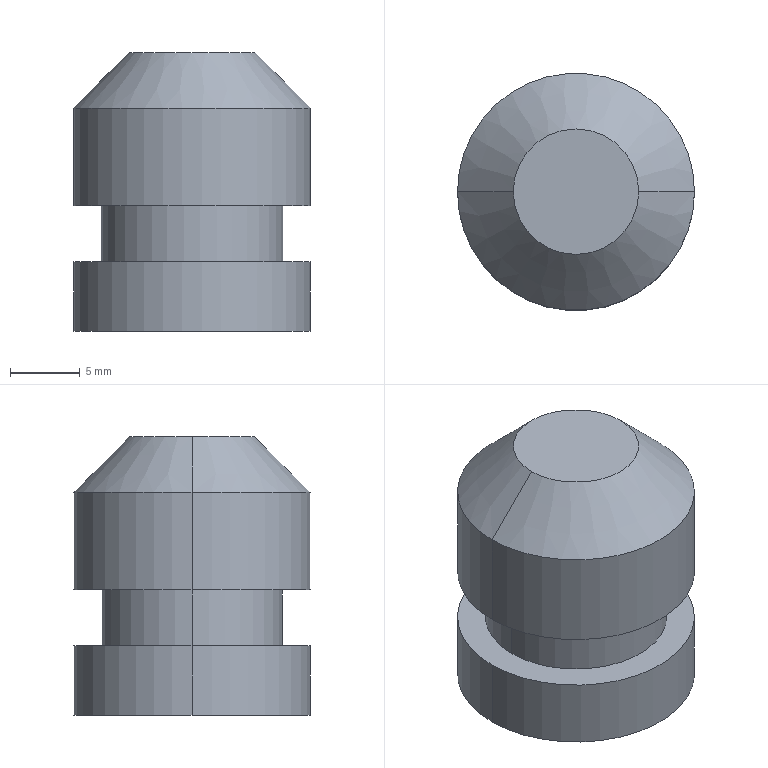Part | SolidWorks | features BaseBody 1 | 1 solid | 18 faces | box 17 x 17 x 20 mm | volume 2436 mm3 | cylinder 8 | cone 4 | plane 4 | sphere 2 | commonest cylinder face diameters 17 x4 10 x2 13 x2
STEP:
#1=CARTESIAN_POINT('',(8.5,0.,16.));
#2=VERTEX_POINT('',#1);
#3=CARTESIAN_POINT('',(8.5,0.,9.));
#4=VERTEX_POINT('',#3);
#5=CARTESIAN_POINT('',(8.5,0.,20.));
#6=DIRECTION('',(0.,0.,-1.));
#7=VECTOR('',#6,1000.);
#8=LINE('',#5,#7);
#9=EDGE_CURVE('',#2,#4,#8,.T.);
#10=ORIENTED_EDGE('',*,*,#9,.F.);
#11=CARTESIAN_POINT('',(-8.5,0.,16.));
#12=VERTEX_POINT('',#11);
#13=CARTESIAN_POINT('',(0.,0.,16.));
#14=DIRECTION('',(0.,0.,-1.));
#15=DIRECTION('',(1.,0.,0.));
#16=AXIS2_PLACEMENT_3D('',#13,#14,#15);
#17=CIRCLE('',#16,8.5);
#18=EDGE_CURVE('',#2,#12,#17,.T.);
#19=ORIENTED_EDGE('',*,*,#18,.T.);
#20=CARTESIAN_POINT('',(-8.5,0.,9.));
#21=VERTEX_POINT('',#20);
#22=CARTESIAN_POINT('',(-8.5,0.,20.));
#23=DIRECTION('',(0.,0.,-1.));
#24=VECTOR('',#23,1000.);
#25=LINE('',#22,#24);
#26=EDGE_CURVE('',#12,#21,#25,.T.);
#27=ORIENTED_EDGE('',*,*,#26,.T.);
#28=CARTESIAN_POINT('',(0.,0.,9.));
#29=DIRECTION('',(0.,0.,1.));
#30=DIRECTION('',(1.,0.,0.));
#31=AXIS2_PLACEMENT_3D('',#28,#29,#30);
#32=CIRCLE('',#31,8.5);
#33=EDGE_CURVE('',#21,#4,#32,.T.);
#34=ORIENTED_EDGE('',*,*,#33,.T.);
#35=EDGE_LOOP('',(#10,#19,#27,#34));
#36=FACE_OUTER_BOUND('',#35,.T.);
#37=CARTESIAN_POINT('',(0.,0.,20.));
#38=DIRECTION('',(0.,0.,-1.));
#39=DIRECTION('',(-1.,0.,0.));
#40=AXIS2_PLACEMENT_3D('',#37,#38,#39);
#41=CYLINDRICAL_SURFACE('',#40,8.5);
#42=ADVANCED_FACE('',(#36),#41,.T.);
#43=CARTESIAN_POINT('',(4.5,0.,20.));
#44=VERTEX_POINT('',#43);
#45=CARTESIAN_POINT('',(4.5,0.,20.));
#46=DIRECTION('',(0.7071,0.,-0.7071));
#47=VECTOR('',#46,1000.);
#48=LINE('',#45,#47);
#49=EDGE_CURVE('',#44,#2,#48,.T.);
#50=ORIENTED_EDGE('',*,*,#49,.F.);
#51=CARTESIAN_POINT('',(-4.5,0.,20.));
#52=VERTEX_POINT('',#51);
#53=CARTESIAN_POINT('',(0.,0.,20.));
#54=DIRECTION('',(0.,0.,1.));
#55=DIRECTION('',(1.,0.,0.));
#56=AXIS2_PLACEMENT_3D('',#53,#54,#55);
#57=CIRCLE('',#56,4.5);
#58=EDGE_CURVE('',#52,#44,#57,.T.);
#59=ORIENTED_EDGE('',*,*,#58,.F.);
#60=CARTESIAN_POINT('',(-4.5,0.,20.));
#61=DIRECTION('',(-0.7071,0.,-0.7071));
#62=VECTOR('',#61,1000.);
#63=LINE('',#60,#62);
#64=EDGE_CURVE('',#52,#12,#63,.T.);
#65=ORIENTED_EDGE('',*,*,#64,.T.);
#66=ORIENTED_EDGE('',*,*,#18,.F.);
#67=EDGE_LOOP('',(#50,#59,#65,#66));
#68=FACE_OUTER_BOUND('',#67,.T.);
#69=CARTESIAN_POINT('',(0.,0.,20.));
#70=DIRECTION('',(0.,0.,-1.));
#71=DIRECTION('',(-1.,0.,0.));
#72=AXIS2_PLACEMENT_3D('',#69,#70,#71);
#73=CONICAL_SURFACE('',#72,4.5,0.7854);
#74=ADVANCED_FACE('',(#68),#73,.T.);
#75=ORIENTED_EDGE('',*,*,#58,.T.);
#76=CARTESIAN_POINT('',(0.,0.,20.));
#77=DIRECTION('',(0.,0.,1.));
#78=DIRECTION('',(1.,0.,0.));
#79=AXIS2_PLACEMENT_3D('',#76,#77,#78);
#80=CIRCLE('',#79,4.5);
#81=EDGE_CURVE('',#44,#52,#80,.T.);
#82=ORIENTED_EDGE('',*,*,#81,.T.);
#83=EDGE_LOOP('',(#75,#82));
#84=FACE_OUTER_BOUND('',#83,.T.);
#85=CARTESIAN_POINT('',(0.,0.,20.));
#86=DIRECTION('',(0.,0.,1.));
#87=DIRECTION('',(1.,0.,0.));
#88=AXIS2_PLACEMENT_3D('',#85,#86,#87);
#89=PLANE('',#88);
#90=ADVANCED_FACE('',(#84),#89,.T.);
#91=CARTESIAN_POINT('',(6.5,0.,9.));
#92=VERTEX_POINT('',#91);
#93=CARTESIAN_POINT('',(6.5,0.,5.));
#94=VERTEX_POINT('',#93);
#95=CARTESIAN_POINT('',(6.5,0.,0.));
#96=DIRECTION('',(0.,0.,-1.));
#97=VECTOR('',#96,1000.);
#98=LINE('',#95,#97);
#99=EDGE_CURVE('',#92,#94,#98,.T.);
#100=ORIENTED_EDGE('',*,*,#99,.F.);
#101=CARTESIAN_POINT('',(-6.5,0.,9.));
#102=VERTEX_POINT('',#101);
#103=CARTESIAN_POINT('',(0.,0.,9.));
#104=DIRECTION('',(0.,0.,-1.));
#105=DIRECTION('',(-1.,0.,0.));
#106=AXIS2_PLACEMENT_3D('',#103,#104,#105);
#107=CIRCLE('',#106,6.5);
#108=EDGE_CURVE('',#92,#102,#107,.T.);
#109=ORIENTED_EDGE('',*,*,#108,.T.);
#110=CARTESIAN_POINT('',(-6.5,0.,5.));
#111=VERTEX_POINT('',#110);
#112=CARTESIAN_POINT('',(-6.5,0.,0.));
#113=DIRECTION('',(0.,0.,-1.));
#114=VECTOR('',#113,1000.);
#115=LINE('',#112,#114);
#116=EDGE_CURVE('',#102,#111,#115,.T.);
#117=ORIENTED_EDGE('',*,*,#116,.T.);
#118=CARTESIAN_POINT('',(0.,0.,5.));
#119=DIRECTION('',(0.,0.,-1.));
#120=DIRECTION('',(-1.,0.,0.));
#121=AXIS2_PLACEMENT_3D('',#118,#119,#120);
#122=CIRCLE('',#121,6.5);
#123=EDGE_CURVE('',#94,#111,#122,.T.);
#124=ORIENTED_EDGE('',*,*,#123,.F.);
#125=EDGE_LOOP('',(#100,#109,#117,#124));
#126=FACE_OUTER_BOUND('',#125,.T.);
#127=CARTESIAN_POINT('',(0.,0.,0.));
#128=DIRECTION('',(0.,0.,-1.));
#129=DIRECTION('',(-1.,0.,0.));
#130=AXIS2_PLACEMENT_3D('',#127,#128,#129);
#131=CYLINDRICAL_SURFACE('',#130,6.5);
#132=ADVANCED_FACE('',(#126),#131,.T.);
#133=CARTESIAN_POINT('',(0.,0.,9.));
#134=DIRECTION('',(0.,0.,-1.));
#135=DIRECTION('',(-1.,0.,0.));
#136=AXIS2_PLACEMENT_3D('',#133,#134,#135);
#137=CIRCLE('',#136,6.5);
#138=EDGE_CURVE('',#102,#92,#137,.T.);
#139=ORIENTED_EDGE('',*,*,#138,.F.);
#140=ORIENTED_EDGE('',*,*,#108,.F.);
#141=EDGE_LOOP('',(#139,#140));
#142=FACE_BOUND('',#141,.T.);
#143=ORIENTED_EDGE('',*,*,#33,.F.);
#144=CARTESIAN_POINT('',(0.,0.,9.));
#145=DIRECTION('',(0.,0.,1.));
#146=DIRECTION('',(1.,0.,0.));
#147=AXIS2_PLACEMENT_3D('',#144,#145,#146);
#148=CIRCLE('',#147,8.5);
#149=EDGE_CURVE('',#4,#21,#148,.T.);
#150=ORIENTED_EDGE('',*,*,#149,.F.);
#151=EDGE_LOOP('',(#143,#150));
#152=FACE_OUTER_BOUND('',#151,.T.);
#153=CARTESIAN_POINT('',(-10.5,0.,9.));
#154=DIRECTION('',(0.,0.,1.));
#155=DIRECTION('',(1.,0.,0.));
#156=AXIS2_PLACEMENT_3D('',#153,#154,#155);
#157=PLANE('',#156);
#158=ADVANCED_FACE('',(#142,#152),#157,.F.);
#159=CARTESIAN_POINT('',(0.,0.,5.));
#160=DIRECTION('',(0.,0.,-1.));
#161=DIRECTION('',(-1.,0.,0.));
#162=AXIS2_PLACEMENT_3D('',#159,#160,#161);
#163=CIRCLE('',#162,6.5);
#164=EDGE_CURVE('',#111,#94,#163,.T.);
#165=ORIENTED_EDGE('',*,*,#164,.T.);
#166=ORIENTED_EDGE('',*,*,#123,.T.);
#167=EDGE_LOOP('',(#165,#166));
#168=FACE_BOUND('',#167,.T.);
#169=CARTESIAN_POINT('',(-8.5,0.,5.));
#170=VERTEX_POINT('',#169);
#171=CARTESIAN_POINT('',(8.5,0.,5.));
#172=VERTEX_POINT('',#171);
#173=CARTESIAN_POINT('',(0.,0.,5.));
#174=DIRECTION('',(0.,0.,-1.));
#175=DIRECTION('',(-1.,0.,0.));
#176=AXIS2_PLACEMENT_3D('',#173,#174,#175);
#177=CIRCLE('',#176,8.5);
#178=EDGE_CURVE('',#170,#172,#177,.T.);
#179=ORIENTED_EDGE('',*,*,#178,.F.);
#180=CARTESIAN_POINT('',(0.,0.,5.));
#181=DIRECTION('',(0.,0.,-1.));
#182=DIRECTION('',(-1.,0.,0.));
#183=AXIS2_PLACEMENT_3D('',#180,#181,#182);
#184=CIRCLE('',#183,8.5);
#185=EDGE_CURVE('',#172,#170,#184,.T.);
#186=ORIENTED_EDGE('',*,*,#185,.F.);
#187=EDGE_LOOP('',(#179,#186));
#188=FACE_OUTER_BOUND('',#187,.T.);
#189=CARTESIAN_POINT('',(-10.5,0.,5.));
#190=DIRECTION('',(0.,0.,-1.));
#191=DIRECTION('',(0.,-1.,0.));
#192=AXIS2_PLACEMENT_3D('',#189,#190,#191);
#193=PLANE('',#192);
#194=ADVANCED_FACE('',(#168,#188),#193,.F.);
#195=CARTESIAN_POINT('',(0.,-5.,13.));
#196=VERTEX_POINT('',#195);
#197=CARTESIAN_POINT('',(0.,5.,13.));
#198=VERTEX_POINT('',#197);
#199=CARTESIAN_POINT('',(0.,0.,13.));
#200=DIRECTION('',(-1.,0.,0.));
#201=DIRECTION('',(0.,-1.,0.));
#202=AXIS2_PLACEMENT_3D('',#199,#200,#201);
#203=CIRCLE('',#202,5.);
#204=EDGE_CURVE('',#196,#198,#203,.T.);
#205=ORIENTED_EDGE('',*,*,#204,.F.);
#206=CARTESIAN_POINT('',(-5.,0.,13.));
#207=VERTEX_POINT('',#206);
#208=CARTESIAN_POINT('',(0.,0.,13.));
#209=DIRECTION('',(0.,0.,1.));
#210=DIRECTION('',(1.,0.,0.));
#211=AXIS2_PLACEMENT_3D('',#208,#209,#210);
#212=CIRCLE('',#211,5.);
#213=EDGE_CURVE('',#207,#196,#212,.T.);
#214=ORIENTED_EDGE('',*,*,#213,.F.);
#215=CARTESIAN_POINT('',(0.,0.,13.));
#216=DIRECTION('',(0.,0.,1.));
#217=DIRECTION('',(1.,0.,0.));
#218=AXIS2_PLACEMENT_3D('',#215,#216,#217);
#219=CIRCLE('',#218,5.);
#220=EDGE_CURVE('',#198,#207,#219,.T.);
#221=ORIENTED_EDGE('',*,*,#220,.F.);
#222=EDGE_LOOP('',(#205,#214,#221));
#223=FACE_OUTER_BOUND('',#222,.T.);
#224=CARTESIAN_POINT('',(0.,0.,13.));
#225=DIRECTION('',(0.,0.,-1.));
#226=DIRECTION('',(0.,1.,0.));
#227=AXIS2_PLACEMENT_3D('',#224,#225,#226);
#228=SPHERICAL_SURFACE('',#227,5.);
#229=ADVANCED_FACE('',(#223),#228,.F.);
#230=CARTESIAN_POINT('',(-5.,0.,5.));
#231=VERTEX_POINT('',#230);
#232=CARTESIAN_POINT('',(-5.,0.,20.));
#233=DIRECTION('',(0.,0.,1.));
#234=VECTOR('',#233,1000.);
#235=LINE('',#232,#234);
#236=EDGE_CURVE('',#231,#207,#235,.T.);
#237=ORIENTED_EDGE('',*,*,#236,.F.);
#238=CARTESIAN_POINT('',(5.,0.,5.));
#239=VERTEX_POINT('',#238);
#240=CARTESIAN_POINT('',(0.,0.,5.));
#241=DIRECTION('',(0.,0.,1.));
#242=DIRECTION('',(1.,0.,0.));
#243=AXIS2_PLACEMENT_3D('',#240,#241,#242);
#244=CIRCLE('',#243,5.);
#245=EDGE_CURVE('',#239,#231,#244,.T.);
#246=ORIENTED_EDGE('',*,*,#245,.F.);
#247=CARTESIAN_POINT('',(5.,0.,13.));
#248=VERTEX_POINT('',#247);
#249=CARTESIAN_POINT('',(5.,0.,20.));
#250=DIRECTION('',(0.,0.,1.));
#251=VECTOR('',#250,1000.);
#252=LINE('',#249,#251);
#253=EDGE_CURVE('',#239,#248,#252,.T.);
#254=ORIENTED_EDGE('',*,*,#253,.T.);
#255=CARTESIAN_POINT('',(0.,0.,13.));
#256=DIRECTION('',(0.,0.,1.));
#257=DIRECTION('',(1.,0.,0.));
#258=AXIS2_PLACEMENT_3D('',#255,#256,#257);
#259=CIRCLE('',#258,5.);
#260=EDGE_CURVE('',#248,#198,#259,.T.);
#261=ORIENTED_EDGE('',*,*,#260,.T.);
#262=ORIENTED_EDGE('',*,*,#220,.T.);
#263=EDGE_LOOP('',(#237,#246,#254,#261,#262));
#264=FACE_OUTER_BOUND('',#263,.T.);
#265=CARTESIAN_POINT('',(0.,0.,20.));
#266=DIRECTION('',(0.,0.,1.));
#267=DIRECTION('',(1.,0.,0.));
#268=AXIS2_PLACEMENT_3D('',#265,#266,#267);
#269=CYLINDRICAL_SURFACE('',#268,5.);
#270=ADVANCED_FACE('',(#264),#269,.F.);
#271=CARTESIAN_POINT('',(6.,0.,0.));
#272=VERTEX_POINT('',#271);
#273=CARTESIAN_POINT('',(6.,0.,0.));
#274=DIRECTION('',(0.1961,0.,-0.9806));
#275=VECTOR('',#274,1000.);
#276=LINE('',#273,#275);
#277=EDGE_CURVE('',#239,#272,#276,.T.);
#278=ORIENTED_EDGE('',*,*,#277,.F.);
#279=ORIENTED_EDGE('',*,*,#245,.T.);
#280=CARTESIAN_POINT('',(-6.,0.,0.));
#281=VERTEX_POINT('',#280);
#282=CARTESIAN_POINT('',(-6.,0.,0.));
#283=DIRECTION('',(-0.1961,0.,-0.9806));
#284=VECTOR('',#283,1000.);
#285=LINE('',#282,#284);
#286=EDGE_CURVE('',#231,#281,#285,.T.);
#287=ORIENTED_EDGE('',*,*,#286,.T.);
#288=CARTESIAN_POINT('',(0.,0.,0.));
#289=DIRECTION('',(0.,0.,1.));
#290=DIRECTION('',(1.,0.,0.));
#291=AXIS2_PLACEMENT_3D('',#288,#289,#290);
#292=CIRCLE('',#291,6.);
#293=EDGE_CURVE('',#272,#281,#292,.T.);
#294=ORIENTED_EDGE('',*,*,#293,.F.);
#295=EDGE_LOOP('',(#278,#279,#287,#294));
#296=FACE_OUTER_BOUND('',#295,.T.);
#297=CARTESIAN_POINT('',(0.,0.,0.));
#298=DIRECTION('',(0.,0.,-1.));
#299=DIRECTION('',(-1.,0.,0.));
#300=AXIS2_PLACEMENT_3D('',#297,#298,#299);
#301=CONICAL_SURFACE('',#300,6.,0.1974);
#302=ADVANCED_FACE('',(#296),#301,.F.);
#303=CARTESIAN_POINT('',(0.,0.,0.));
#304=DIRECTION('',(0.,0.,1.));
#305=DIRECTION('',(1.,0.,0.));
#306=AXIS2_PLACEMENT_3D('',#303,#304,#305);
#307=CIRCLE('',#306,6.);
#308=EDGE_CURVE('',#281,#272,#307,.T.);
#309=ORIENTED_EDGE('',*,*,#308,.T.);
#310=ORIENTED_EDGE('',*,*,#293,.T.);
#311=EDGE_LOOP('',(#309,#310));
#312=FACE_BOUND('',#311,.T.);
#313=CARTESIAN_POINT('',(-8.5,0.,0.));
#314=VERTEX_POINT('',#313);
#315=CARTESIAN_POINT('',(8.5,0.,0.));
#316=VERTEX_POINT('',#315);
#317=CARTESIAN_POINT('',(0.,0.,0.));
#318=DIRECTION('',(0.,0.,1.));
#319=DIRECTION('',(1.,0.,0.));
#320=AXIS2_PLACEMENT_3D('',#317,#318,#319);
#321=CIRCLE('',#320,8.5);
#322=EDGE_CURVE('',#314,#316,#321,.T.);
#323=ORIENTED_EDGE('',*,*,#322,.F.);
#324=CARTESIAN_POINT('',(0.,0.,0.));
#325=DIRECTION('',(0.,0.,1.));
#326=DIRECTION('',(1.,0.,0.));
#327=AXIS2_PLACEMENT_3D('',#324,#325,#326);
#328=CIRCLE('',#327,8.5);
#329=EDGE_CURVE('',#316,#314,#328,.T.);
#330=ORIENTED_EDGE('',*,*,#329,.F.);
#331=EDGE_LOOP('',(#323,#330));
#332=FACE_OUTER_BOUND('',#331,.T.);
#333=CARTESIAN_POINT('',(0.,0.,0.));
#334=DIRECTION('',(0.,0.,1.));
#335=DIRECTION('',(1.,0.,0.));
#336=AXIS2_PLACEMENT_3D('',#333,#334,#335);
#337=PLANE('',#336);
#338=ADVANCED_FACE('',(#312,#332),#337,.F.);
#339=CARTESIAN_POINT('',(8.5,0.,20.));
#340=DIRECTION('',(0.,0.,-1.));
#341=VECTOR('',#340,1000.);
#342=LINE('',#339,#341);
#343=EDGE_CURVE('',#172,#316,#342,.T.);
#344=ORIENTED_EDGE('',*,*,#343,.F.);
#345=ORIENTED_EDGE('',*,*,#185,.T.);
#346=CARTESIAN_POINT('',(-8.5,0.,20.));
#347=DIRECTION('',(0.,0.,-1.));
#348=VECTOR('',#347,1000.);
#349=LINE('',#346,#348);
#350=EDGE_CURVE('',#170,#314,#349,.T.);
#351=ORIENTED_EDGE('',*,*,#350,.T.);
#352=ORIENTED_EDGE('',*,*,#322,.T.);
#353=EDGE_LOOP('',(#344,#345,#351,#352));
#354=FACE_OUTER_BOUND('',#353,.T.);
#355=CARTESIAN_POINT('',(0.,0.,20.));
#356=DIRECTION('',(0.,0.,-1.));
#357=DIRECTION('',(-1.,0.,0.));
#358=AXIS2_PLACEMENT_3D('',#355,#356,#357);
#359=CYLINDRICAL_SURFACE('',#358,8.5);
#360=ADVANCED_FACE('',(#354),#359,.T.);
#361=ORIENTED_EDGE('',*,*,#178,.T.);
#362=ORIENTED_EDGE('',*,*,#343,.T.);
#363=ORIENTED_EDGE('',*,*,#329,.T.);
#364=ORIENTED_EDGE('',*,*,#350,.F.);
#365=EDGE_LOOP('',(#361,#362,#363,#364));
#366=FACE_OUTER_BOUND('',#365,.T.);
#367=CARTESIAN_POINT('',(0.,0.,20.));
#368=DIRECTION('',(0.,0.,-1.));
#369=DIRECTION('',(-1.,0.,0.));
#370=AXIS2_PLACEMENT_3D('',#367,#368,#369);
#371=CYLINDRICAL_SURFACE('',#370,8.5);
#372=ADVANCED_FACE('',(#366),#371,.T.);
#373=CARTESIAN_POINT('',(0.,0.,5.));
#374=DIRECTION('',(0.,0.,1.));
#375=DIRECTION('',(1.,0.,0.));
#376=AXIS2_PLACEMENT_3D('',#373,#374,#375);
#377=CIRCLE('',#376,5.);
#378=EDGE_CURVE('',#231,#239,#377,.T.);
#379=ORIENTED_EDGE('',*,*,#378,.T.);
#380=ORIENTED_EDGE('',*,*,#277,.T.);
#381=ORIENTED_EDGE('',*,*,#308,.F.);
#382=ORIENTED_EDGE('',*,*,#286,.F.);
#383=EDGE_LOOP('',(#379,#380,#381,#382));
#384=FACE_OUTER_BOUND('',#383,.T.);
#385=CARTESIAN_POINT('',(0.,0.,0.));
#386=DIRECTION('',(0.,0.,-1.));
#387=DIRECTION('',(-1.,0.,0.));
#388=AXIS2_PLACEMENT_3D('',#385,#386,#387);
#389=CONICAL_SURFACE('',#388,6.,0.1974);
#390=ADVANCED_FACE('',(#384),#389,.F.);
#391=ORIENTED_EDGE('',*,*,#378,.F.);
#392=ORIENTED_EDGE('',*,*,#236,.T.);
#393=ORIENTED_EDGE('',*,*,#213,.T.);
#394=CARTESIAN_POINT('',(0.,0.,13.));
#395=DIRECTION('',(0.,0.,1.));
#396=DIRECTION('',(1.,0.,0.));
#397=AXIS2_PLACEMENT_3D('',#394,#395,#396);
#398=CIRCLE('',#397,5.);
#399=EDGE_CURVE('',#196,#248,#398,.T.);
#400=ORIENTED_EDGE('',*,*,#399,.T.);
#401=ORIENTED_EDGE('',*,*,#253,.F.);
#402=EDGE_LOOP('',(#391,#392,#393,#400,#401));
#403=FACE_OUTER_BOUND('',#402,.T.);
#404=CARTESIAN_POINT('',(0.,0.,20.));
#405=DIRECTION('',(0.,0.,1.));
#406=DIRECTION('',(1.,0.,0.));
#407=AXIS2_PLACEMENT_3D('',#404,#405,#406);
#408=CYLINDRICAL_SURFACE('',#407,5.);
#409=ADVANCED_FACE('',(#403),#408,.F.);
#410=ORIENTED_EDGE('',*,*,#399,.F.);
#411=ORIENTED_EDGE('',*,*,#204,.T.);
#412=ORIENTED_EDGE('',*,*,#260,.F.);
#413=EDGE_LOOP('',(#410,#411,#412));
#414=FACE_OUTER_BOUND('',#413,.T.);
#415=CARTESIAN_POINT('',(0.,0.,13.));
#416=DIRECTION('',(0.,0.,-1.));
#417=DIRECTION('',(0.,1.,0.));
#418=AXIS2_PLACEMENT_3D('',#415,#416,#417);
#419=SPHERICAL_SURFACE('',#418,5.);
#420=ADVANCED_FACE('',(#414),#419,.F.);
#421=ORIENTED_EDGE('',*,*,#138,.T.);
#422=ORIENTED_EDGE('',*,*,#99,.T.);
#423=ORIENTED_EDGE('',*,*,#164,.F.);
#424=ORIENTED_EDGE('',*,*,#116,.F.);
#425=EDGE_LOOP('',(#421,#422,#423,#424));
#426=FACE_OUTER_BOUND('',#425,.T.);
#427=CARTESIAN_POINT('',(0.,0.,0.));
#428=DIRECTION('',(0.,0.,-1.));
#429=DIRECTION('',(-1.,0.,0.));
#430=AXIS2_PLACEMENT_3D('',#427,#428,#429);
#431=CYLINDRICAL_SURFACE('',#430,6.5);
#432=ADVANCED_FACE('',(#426),#431,.T.);
#433=ORIENTED_EDGE('',*,*,#81,.F.);
#434=ORIENTED_EDGE('',*,*,#49,.T.);
#435=CARTESIAN_POINT('',(0.,0.,16.));
#436=DIRECTION('',(0.,0.,-1.));
#437=DIRECTION('',(1.,0.,0.));
#438=AXIS2_PLACEMENT_3D('',#435,#436,#437);
#439=CIRCLE('',#438,8.5);
#440=EDGE_CURVE('',#12,#2,#439,.T.);
#441=ORIENTED_EDGE('',*,*,#440,.F.);
#442=ORIENTED_EDGE('',*,*,#64,.F.);
#443=EDGE_LOOP('',(#433,#434,#441,#442));
#444=FACE_OUTER_BOUND('',#443,.T.);
#445=CARTESIAN_POINT('',(0.,0.,20.));
#446=DIRECTION('',(0.,0.,-1.));
#447=DIRECTION('',(-1.,0.,0.));
#448=AXIS2_PLACEMENT_3D('',#445,#446,#447);
#449=CONICAL_SURFACE('',#448,4.5,0.7854);
#450=ADVANCED_FACE('',(#444),#449,.T.);
#451=ORIENTED_EDGE('',*,*,#440,.T.);
#452=ORIENTED_EDGE('',*,*,#9,.T.);
#453=ORIENTED_EDGE('',*,*,#149,.T.);
#454=ORIENTED_EDGE('',*,*,#26,.F.);
#455=EDGE_LOOP('',(#451,#452,#453,#454));
#456=FACE_OUTER_BOUND('',#455,.T.);
#457=CARTESIAN_POINT('',(0.,0.,20.));
#458=DIRECTION('',(0.,0.,-1.));
#459=DIRECTION('',(-1.,0.,0.));
#460=AXIS2_PLACEMENT_3D('',#457,#458,#459);
#461=CYLINDRICAL_SURFACE('',#460,8.5);
#462=ADVANCED_FACE('',(#456),#461,.T.);
#463=CLOSED_SHELL('',(#42,#74,#90,#132,#158,#194,#229,#270,#302,#338,#360,#372,#390,#409,#420,#432,#450,#462));
#464=MANIFOLD_SOLID_BREP('',#463);
#465=CARTESIAN_POINT('',(0.,0.,0.));
#466=DIRECTION('',(0.,0.,1.));
#467=DIRECTION('',(1.,0.,0.));
#468=AXIS2_PLACEMENT_3D('',#465,#466,#467);
#469=(LENGTH_UNIT()NAMED_UNIT(*)SI_UNIT(.MILLI.,.METRE.));
#470=UNCERTAINTY_MEASURE_WITH_UNIT(LENGTH_MEASURE(0.00001),#469,'','');
#471=(NAMED_UNIT(*)PLANE_ANGLE_UNIT()SI_UNIT($,.RADIAN.));
#472=(NAMED_UNIT(*)SI_UNIT($,.STERADIAN.)SOLID_ANGLE_UNIT());
#473=(GEOMETRIC_REPRESENTATION_CONTEXT(3)GLOBAL_UNCERTAINTY_ASSIGNED_CONTEXT((#470))GLOBAL_UNIT_ASSIGNED_CONTEXT((#469,#471,#472))REPRESENTATION_CONTEXT('',''));
#474=ADVANCED_BREP_SHAPE_REPRESENTATION('',(#464,#468),#473);